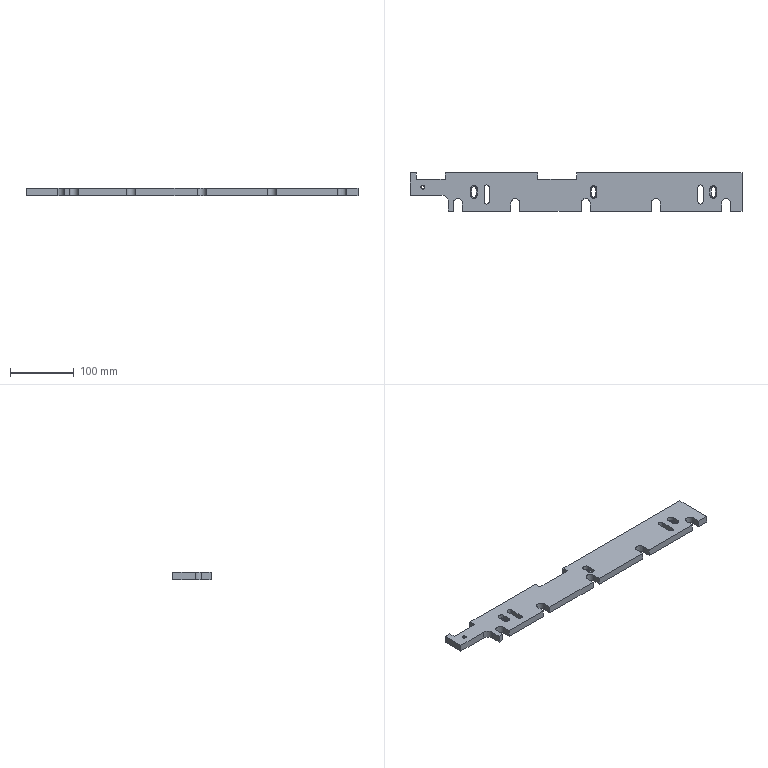Part | STEP file | Tube feed_id950_x_t | 1 solid | 93 faces | box 520 x 59.75 x 11 mm | volume 287965 mm3 | plane 50 | cylinder 29 | cone 14 | commonest cylinder face diameters 4.2 x6 6.8 x6 10.5 x6 14 x5 8 x4 5 x1